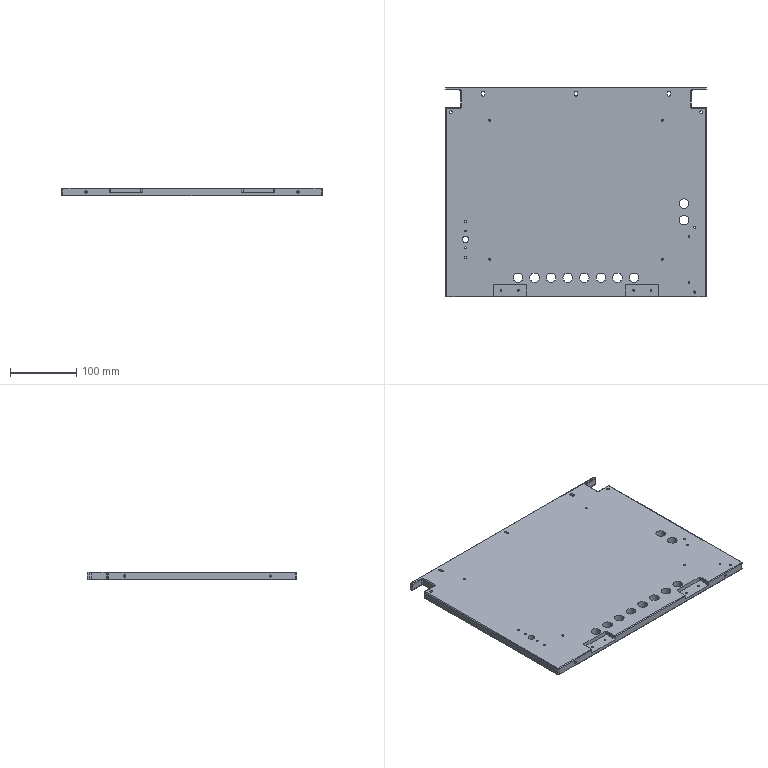Part | 1 solid | 165 faces | box 393.6 x 317 x 12 mm | volume 880470 mm3 | cylinder 93 | plane 42 | sphere 12 | torus 12 | cone 6 | commonest cylinder face diameters 2 x32 3.3 x14 4 x10 14.5 x10 2.5 x8 4.5 x6